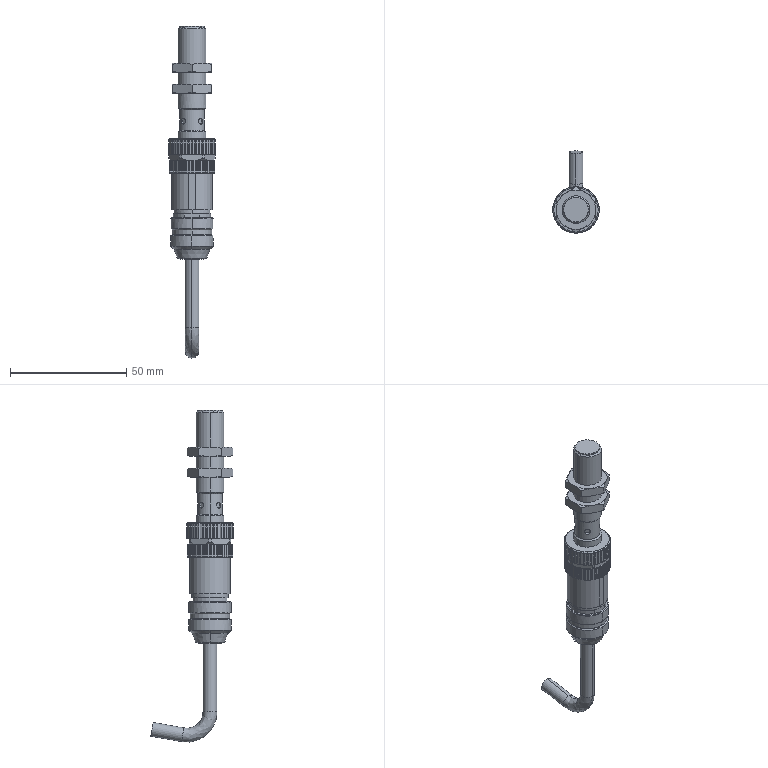Part | SolidWorks | features BaseBody 2 | 2 solids | 659 faces | box 20 x 35.517 x 143.072 mm | volume 16488 mm3 | plane 350 | cylinder 187 | cone 120 | spline 2 | commonest cylinder face diameters 19.5 x50 20 x38 2.5 x12 12 x10 1 x8 1.1 x8